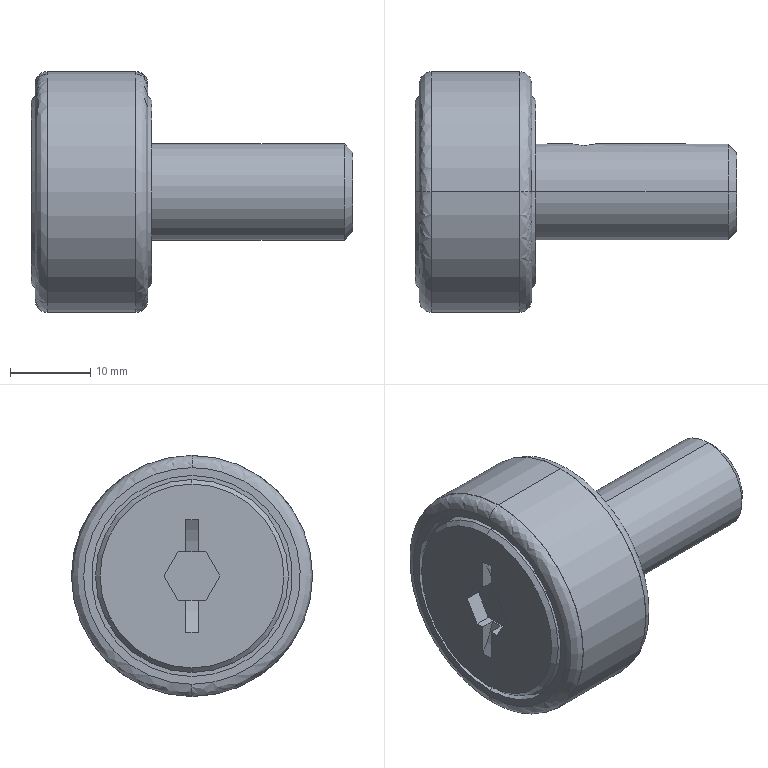Part | STEP file | PN_0073_default | 1 solid | 56 faces | box 40 x 30 x 30 mm | volume 12542 mm3 | cylinder 21 | plane 21 | cone 10 | spline 4 | commonest cylinder face diameters 3 x5 24 x4 25 x4 6 x2 12 x2 20 x2